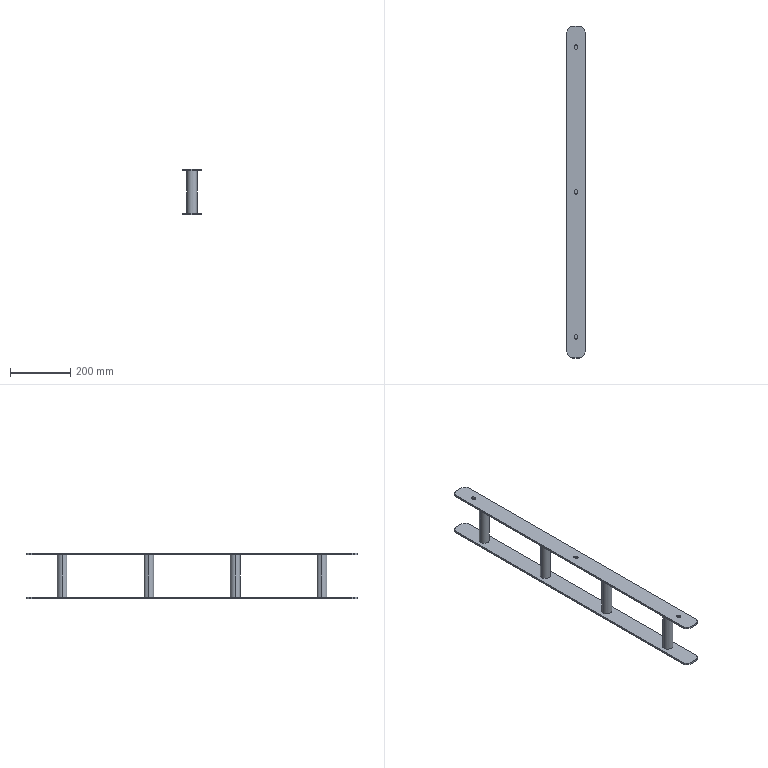Part | SolidWorks | 6 solids | 56 faces | box 60 x 1100 x 152 mm | volume 992973 mm3 | cylinder 30 | plane 26 | commonest cylinder face diameters 25.5 x8 33.5 x8 40 x8 11 x6